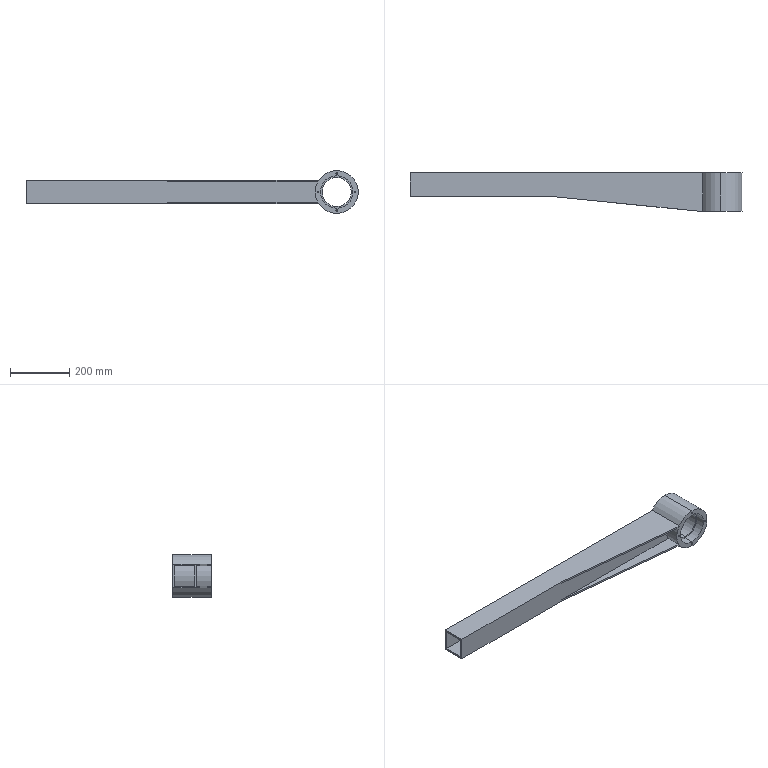Part | SolidWorks | features CirPattern 2, HoleWzd 2, ICE 2, MirrorPattern 1, Revolution 1, Shell 1 | 1 solid | 59 faces | box 1122 x 130 x 145 mm | volume 2935310 mm3 | cylinder 27 | cone 16 | plane 16 | commonest cylinder face diameters 5 x16 145 x5 110 x4 99 x2